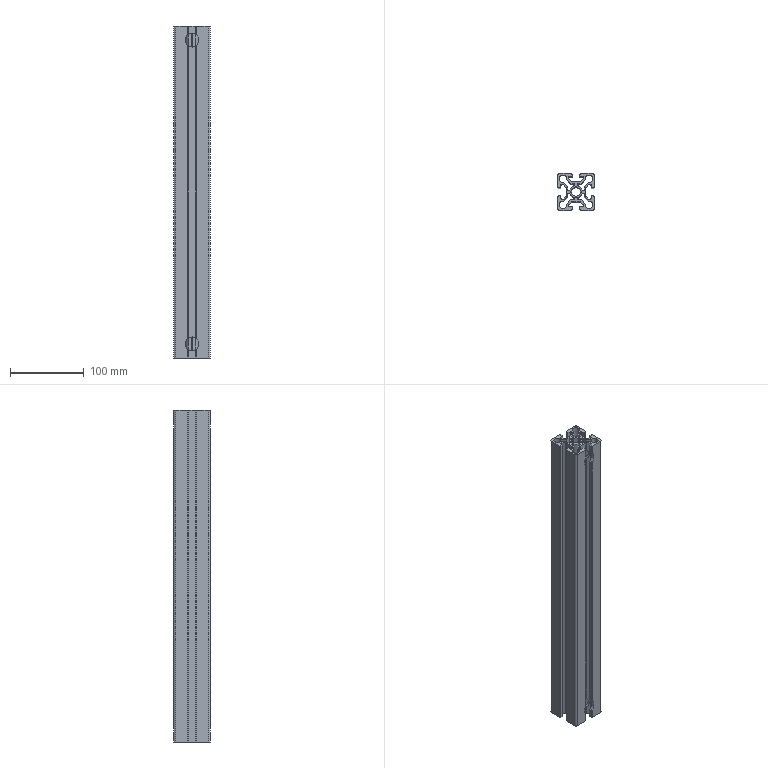Part | NX | features BREP 1 | 1 solid | 231 faces | box 50 x 50 x 450 mm | volume 439698 mm3 | plane 154 | cylinder 77 | commonest cylinder face diameters 2 x37 19 x16 10 x12 6 x4 12 x4 17 x4